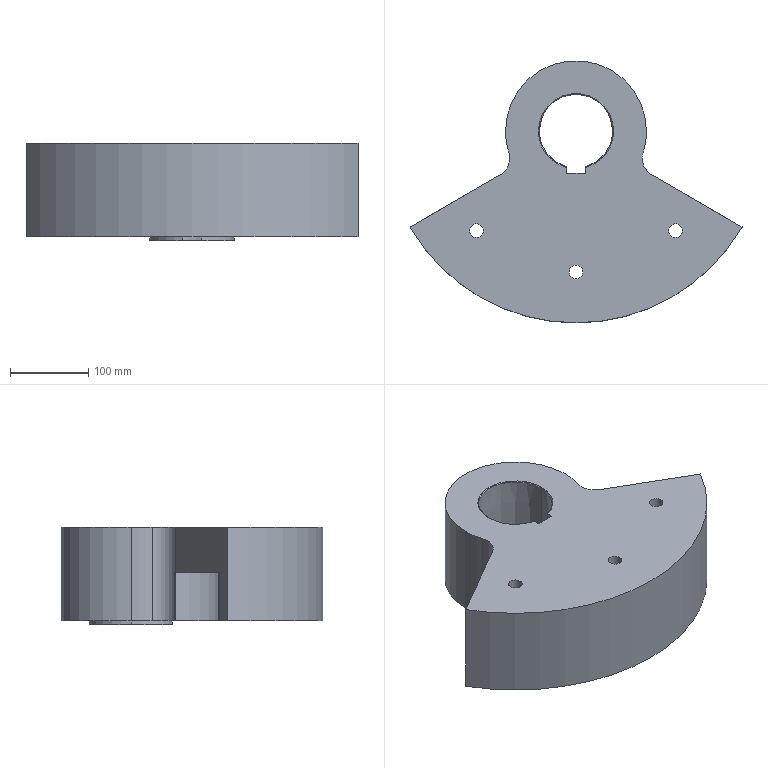Part | STEP file | Offset block | 1 solid | 55 faces | box 424.352 x 335 x 125 mm | volume 6174570 mm3 | cylinder 26 | cone 17 | plane 12 | commonest cylinder face diameters 17.5 x14 50 x3 108 x3 180 x3 224 x1 450 x1